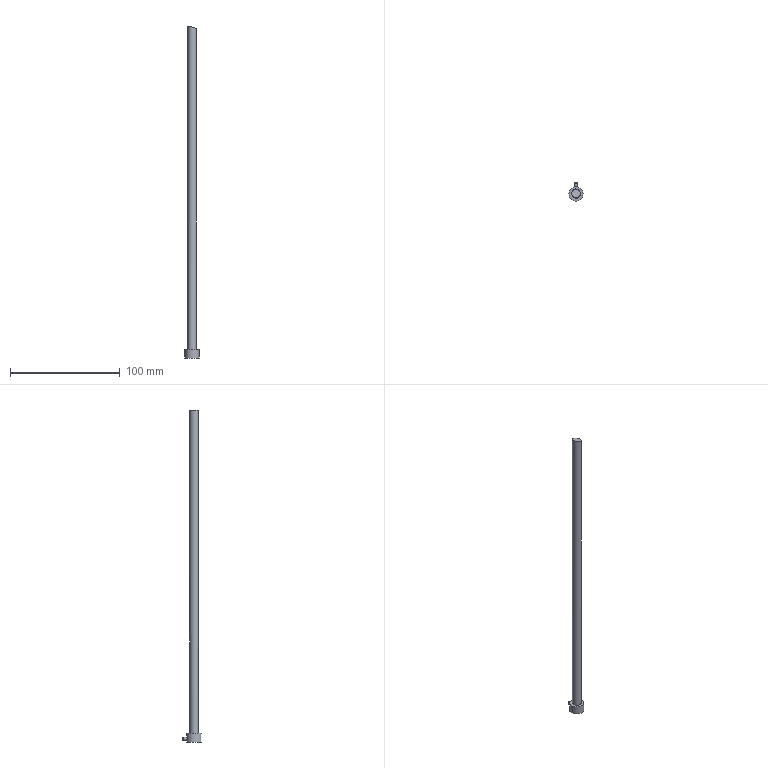Part | STEP file | E108-08-310 | 1 solid | 8 faces | box 13 x 16.5 x 302.869 mm | volume 15847 mm3 | cylinder 3 | plane 3 | spline 1 | cone 1 | commonest cylinder face diameters 3 x1 8 x1 13 x1
STEP:
#1=CARTESIAN_POINT('',(0.,0.,0.));
#2=DIRECTION('',(0.,0.,1.));
#3=DIRECTION('',(1.,0.,0.));
#4=AXIS2_PLACEMENT_3D('',#1,#2,#3);
#5=CARTESIAN_POINT('',(3.978,0.4166,300.445));
#6=VERTEX_POINT('',#5);
#7=CARTESIAN_POINT('',(3.978,0.4166,300.445));
#8=CARTESIAN_POINT('',(3.933,0.8473,300.446));
#9=CARTESIAN_POINT('',(3.815,1.276,300.47));
#10=CARTESIAN_POINT('',(3.636,1.668,300.514));
#11=CARTESIAN_POINT('',(3.456,2.059,300.558));
#12=CARTESIAN_POINT('',(3.21,2.424,300.623));
#13=CARTESIAN_POINT('',(2.92,2.734,300.703));
#14=CARTESIAN_POINT('',(2.623,3.051,300.785));
#15=CARTESIAN_POINT('',(2.272,3.319,300.885));
#16=CARTESIAN_POINT('',(1.896,3.522,300.994));
#17=CARTESIAN_POINT('',(1.503,3.734,301.108));
#18=CARTESIAN_POINT('',(1.071,3.879,301.235));
#19=CARTESIAN_POINT('',(0.6351,3.949,301.365));
#20=CARTESIAN_POINT('',(0.1817,4.022,301.5));
#21=CARTESIAN_POINT('',(-0.289,4.016,301.642));
#22=CARTESIAN_POINT('',(-0.7396,3.931,301.779));
#23=CARTESIAN_POINT('',(-1.199,3.845,301.92));
#24=CARTESIAN_POINT('',(-1.65,3.674,302.059));
#25=CARTESIAN_POINT('',(-2.054,3.432,302.186));
#26=CARTESIAN_POINT('',(-2.455,3.193,302.312));
#27=CARTESIAN_POINT('',(-2.82,2.876,302.43));
#28=CARTESIAN_POINT('',(-3.117,2.507,302.528));
#29=CARTESIAN_POINT('',(-3.404,2.15,302.623));
#30=CARTESIAN_POINT('',(-3.634,1.734,302.703));
#31=CARTESIAN_POINT('',(-3.785,1.295,302.76));
#32=CARTESIAN_POINT('',(-3.929,0.8741,302.815));
#33=CARTESIAN_POINT('',(-4.003,0.4197,302.851));
#34=CARTESIAN_POINT('',(-4.,-0.02828,302.863));
#35=CARTESIAN_POINT('',(-3.997,-0.4621,302.876));
#36=CARTESIAN_POINT('',(-3.921,-0.9021,302.867));
#37=CARTESIAN_POINT('',(-3.779,-1.311,302.838));
#38=CARTESIAN_POINT('',(-3.638,-1.717,302.809));
#39=CARTESIAN_POINT('',(-3.429,-2.103,302.76));
#40=CARTESIAN_POINT('',(-3.17,-2.44,302.694));
#41=CARTESIAN_POINT('',(-2.906,-2.782,302.627));
#42=CARTESIAN_POINT('',(-2.584,-3.083,302.541));
#43=CARTESIAN_POINT('',(-2.23,-3.32,302.444));
#44=CARTESIAN_POINT('',(-1.864,-3.567,302.343));
#45=CARTESIAN_POINT('',(-1.454,-3.752,302.227));
#46=CARTESIAN_POINT('',(-1.033,-3.864,302.104));
#47=CARTESIAN_POINT('',(-0.5946,-3.982,301.977));
#48=CARTESIAN_POINT('',(-0.1325,-4.023,301.839));
#49=CARTESIAN_POINT('',(0.317,-3.987,301.702));
#50=CARTESIAN_POINT('',(0.78,-3.951,301.561));
#51=CARTESIAN_POINT('',(1.242,-3.831,301.417));
#52=CARTESIAN_POINT('',(1.666,-3.636,301.282));
#53=CARTESIAN_POINT('',(2.092,-3.441,301.146));
#54=CARTESIAN_POINT('',(2.491,-3.165,301.015));
#55=CARTESIAN_POINT('',(2.827,-2.83,300.901));
#56=CARTESIAN_POINT('',(3.154,-2.503,300.79));
#57=CARTESIAN_POINT('',(3.431,-2.11,300.692));
#58=CARTESIAN_POINT('',(3.629,-1.683,300.618));
#59=CARTESIAN_POINT('',(3.818,-1.276,300.547));
#60=CARTESIAN_POINT('',(3.94,-0.8259,300.495));
#61=CARTESIAN_POINT('',(3.983,-0.3737,300.468));
#62=CARTESIAN_POINT('',(4.007,-0.1118,300.453));
#63=CARTESIAN_POINT('',(4.006,0.1545,300.445));
#64=CARTESIAN_POINT('',(3.978,0.4166,300.445));
#65=B_SPLINE_CURVE_WITH_KNOTS('',3,(#7,#8,#9,#10,#11,#12,#13,#14,#15,#16,#17,#18,#19,#20,#21,#22,#23,#24,#25,#26,#27,#28,#29,#30,#31,#32,#33,#34,#35,#36,#37,#38,#39,#40,#41,#42,#43,#44,#45,#46,#47,#48,#49,#50,#51,#52,#53,#54,#55,#56,#57,#58,#59,#60,#61,#62,#63,#64),.UNSPECIFIED.,.T.,.F.,(1,3,3,3,3,3,3,3,3,3,3,3,3,3,3,3,3,3,3,3,3,1),(-0.03062,0.,0.05078,0.1015,0.1532,0.2072,0.2634,0.3207,0.3775,0.4324,0.485,0.5359,0.5863,0.6375,0.6906,0.7458,0.8028,0.8601,0.916,0.9694,1.,1.051),.UNSPECIFIED.);
#66=CARTESIAN_POINT('',(0.,0.,108.));
#67=DIRECTION('',(0.,0.,-1.));
#68=DIRECTION('',(-1.,0.,0.));
#69=AXIS2_PLACEMENT_3D('',#66,#67,#68);
#70=CYLINDRICAL_SURFACE('',#69,4.);
#71=CARTESIAN_POINT('',(9.32,-192.445));
#72=CARTESIAN_POINT('',(9.296,-192.446));
#73=CARTESIAN_POINT('',(9.248,-192.448));
#74=CARTESIAN_POINT('',(9.174,-192.459));
#75=CARTESIAN_POINT('',(9.101,-192.476));
#76=CARTESIAN_POINT('',(9.029,-192.5));
#77=CARTESIAN_POINT('',(8.956,-192.529));
#78=CARTESIAN_POINT('',(8.884,-192.565));
#79=CARTESIAN_POINT('',(8.811,-192.607));
#80=CARTESIAN_POINT('',(8.739,-192.654));
#81=CARTESIAN_POINT('',(8.667,-192.706));
#82=CARTESIAN_POINT('',(8.596,-192.763));
#83=CARTESIAN_POINT('',(8.524,-192.824));
#84=CARTESIAN_POINT('',(8.453,-192.89));
#85=CARTESIAN_POINT('',(8.382,-192.959));
#86=CARTESIAN_POINT('',(8.311,-193.031));
#87=CARTESIAN_POINT('',(8.241,-193.106));
#88=CARTESIAN_POINT('',(8.17,-193.184));
#89=CARTESIAN_POINT('',(8.1,-193.264));
#90=CARTESIAN_POINT('',(8.03,-193.345));
#91=CARTESIAN_POINT('',(7.96,-193.427));
#92=CARTESIAN_POINT('',(7.89,-193.511));
#93=CARTESIAN_POINT('',(7.82,-193.596));
#94=CARTESIAN_POINT('',(7.75,-193.68));
#95=CARTESIAN_POINT('',(7.68,-193.765));
#96=CARTESIAN_POINT('',(7.611,-193.848));
#97=CARTESIAN_POINT('',(7.541,-193.931));
#98=CARTESIAN_POINT('',(7.471,-194.012));
#99=CARTESIAN_POINT('',(7.4,-194.092));
#100=CARTESIAN_POINT('',(7.33,-194.17));
#101=CARTESIAN_POINT('',(7.26,-194.245));
#102=CARTESIAN_POINT('',(7.189,-194.318));
#103=CARTESIAN_POINT('',(7.118,-194.387));
#104=CARTESIAN_POINT('',(7.047,-194.453));
#105=CARTESIAN_POINT('',(6.976,-194.516));
#106=CARTESIAN_POINT('',(6.905,-194.574));
#107=CARTESIAN_POINT('',(6.833,-194.627));
#108=CARTESIAN_POINT('',(6.761,-194.677));
#109=CARTESIAN_POINT('',(6.688,-194.721));
#110=CARTESIAN_POINT('',(6.616,-194.759));
#111=CARTESIAN_POINT('',(6.544,-194.792));
#112=CARTESIAN_POINT('',(6.471,-194.82));
#113=CARTESIAN_POINT('',(6.398,-194.842));
#114=CARTESIAN_POINT('',(6.325,-194.857));
#115=CARTESIAN_POINT('',(6.253,-194.867));
#116=CARTESIAN_POINT('',(6.18,-194.87));
#117=CARTESIAN_POINT('',(6.106,-194.867));
#118=CARTESIAN_POINT('',(6.033,-194.857));
#119=CARTESIAN_POINT('',(5.96,-194.842));
#120=CARTESIAN_POINT('',(5.888,-194.82));
#121=CARTESIAN_POINT('',(5.815,-194.793));
#122=CARTESIAN_POINT('',(5.742,-194.759));
#123=CARTESIAN_POINT('',(5.67,-194.72));
#124=CARTESIAN_POINT('',(5.598,-194.676));
#125=CARTESIAN_POINT('',(5.526,-194.627));
#126=CARTESIAN_POINT('',(5.454,-194.573));
#127=CARTESIAN_POINT('',(5.382,-194.514));
#128=CARTESIAN_POINT('',(5.311,-194.451));
#129=CARTESIAN_POINT('',(5.24,-194.385));
#130=CARTESIAN_POINT('',(5.169,-194.314));
#131=CARTESIAN_POINT('',(5.098,-194.241));
#132=CARTESIAN_POINT('',(5.028,-194.165));
#133=CARTESIAN_POINT('',(4.958,-194.087));
#134=CARTESIAN_POINT('',(4.887,-194.006));
#135=CARTESIAN_POINT('',(4.817,-193.924));
#136=CARTESIAN_POINT('',(4.747,-193.84));
#137=CARTESIAN_POINT('',(4.677,-193.756));
#138=CARTESIAN_POINT('',(4.608,-193.672));
#139=CARTESIAN_POINT('',(4.538,-193.587));
#140=CARTESIAN_POINT('',(4.468,-193.502));
#141=CARTESIAN_POINT('',(4.398,-193.417));
#142=CARTESIAN_POINT('',(4.328,-193.334));
#143=CARTESIAN_POINT('',(4.258,-193.253));
#144=CARTESIAN_POINT('',(4.188,-193.173));
#145=CARTESIAN_POINT('',(4.118,-193.095));
#146=CARTESIAN_POINT('',(4.047,-193.02));
#147=CARTESIAN_POINT('',(3.976,-192.948));
#148=CARTESIAN_POINT('',(3.906,-192.879));
#149=CARTESIAN_POINT('',(3.835,-192.814));
#150=CARTESIAN_POINT('',(3.763,-192.754));
#151=CARTESIAN_POINT('',(3.691,-192.697));
#152=CARTESIAN_POINT('',(3.619,-192.646));
#153=CARTESIAN_POINT('',(3.548,-192.6));
#154=CARTESIAN_POINT('',(3.475,-192.559));
#155=CARTESIAN_POINT('',(3.403,-192.524));
#156=CARTESIAN_POINT('',(3.33,-192.495));
#157=CARTESIAN_POINT('',(3.257,-192.473));
#158=CARTESIAN_POINT('',(3.184,-192.457));
#159=CARTESIAN_POINT('',(3.111,-192.447));
#160=CARTESIAN_POINT('',(3.062,-192.445));
#161=CARTESIAN_POINT('',(3.037,-192.445));
#162=B_SPLINE_CURVE_WITH_KNOTS('',3,(#71,#72,#73,#74,#75,#76,#77,#78,#79,#80,#81,#82,#83,#84,#85,#86,#87,#88,#89,#90,#91,#92,#93,#94,#95,#96,#97,#98,#99,#100,#101,#102,#103,#104,#105,#106,#107,#108,#109,#110,#111,#112,#113,#114,#115,#116,#117,#118,#119,#120,#121,#122,#123,#124,#125,#126,#127,#128,#129,#130,#131,#132,#133,#134,#135,#136,#137,#138,#139,#140,#141,#142,#143,#144,#145,#146,#147,#148,#149,#150,#151,#152,#153,#154,#155,#156,#157,#158,#159,#160,#161),.UNSPECIFIED.,.F.,.F.,(4,1,1,1,1,1,1,1,1,1,1,1,1,1,1,1,1,1,1,1,1,1,1,1,1,1,1,1,1,1,1,1,1,1,1,1,1,1,1,1,1,1,1,1,1,1,1,1,1,1,1,1,1,1,1,1,1,1,1,1,1,1,1,1,1,1,1,1,1,1,1,1,1,1,1,1,1,1,1,1,1,1,1,1,1,1,1,1,4),(0.,0.01136,0.02273,0.03409,0.04545,0.05682,0.06818,0.07955,0.09091,0.1023,0.1136,0.125,0.1364,0.1477,0.1591,0.1705,0.1818,0.1932,0.2045,0.2159,0.2273,0.2386,0.25,0.2614,0.2727,0.2841,0.2955,0.3068,0.3182,0.3295,0.3409,0.3523,0.3636,0.375,0.3864,0.3977,0.4091,0.4205,0.4318,0.4432,0.4545,0.4659,0.4773,0.4886,0.5,0.5114,0.5227,0.5341,0.5455,0.5568,0.5682,0.5795,0.5909,0.6023,0.6136,0.625,0.6364,0.6477,0.6591,0.6705,0.6818,0.6932,0.7045,0.7159,0.7273,0.7386,0.75,0.7614,0.7727,0.7841,0.7955,0.8068,0.8182,0.8295,0.8409,0.8523,0.8636,0.875,0.8864,0.8977,0.9091,0.9205,0.9318,0.9432,0.9545,0.9659,0.9773,0.9886,1.),.QUASI_UNIFORM_KNOTS.);
#163=(GEOMETRIC_REPRESENTATION_CONTEXT(2)PARAMETRIC_REPRESENTATION_CONTEXT()REPRESENTATION_CONTEXT('',''));
#164=DEFINITIONAL_REPRESENTATION('',(#162),#163);
#165=PCURVE('',#70,#164);
#166=CARTESIAN_POINT('',(-6.093,-7.25,303.685));
#167=CARTESIAN_POINT('',(-0.8456,-7.248,302.186));
#168=CARTESIAN_POINT('',(4.462,-7.246,300.56));
#169=CARTESIAN_POINT('',(9.83,-7.244,298.812));
#170=CARTESIAN_POINT('',(-6.112,-2.699,303.554));
#171=CARTESIAN_POINT('',(-0.8669,-2.697,302.056));
#172=CARTESIAN_POINT('',(4.438,-2.695,300.432));
#173=CARTESIAN_POINT('',(9.803,-2.692,298.685));
#174=CARTESIAN_POINT('',(-6.133,1.852,303.422));
#175=CARTESIAN_POINT('',(-0.8912,1.854,301.925));
#176=CARTESIAN_POINT('',(4.411,1.856,300.302));
#177=CARTESIAN_POINT('',(9.773,1.859,298.557));
#178=CARTESIAN_POINT('',(-6.157,6.403,303.288));
#179=CARTESIAN_POINT('',(-0.9182,6.405,301.793));
#180=CARTESIAN_POINT('',(4.381,6.407,300.171));
#181=CARTESIAN_POINT('',(9.741,6.409,298.427));
#182=B_SPLINE_SURFACE_WITH_KNOTS('',3,3,((#166,#167,#168,#169),(#170,#171,#172,#173),(#174,#175,#176,#177),(#178,#179,#180,#181)),.UNSPECIFIED.,.F.,.F.,.F.,(4,4),(4,4),(0.,1.),(0.,1.),.PIECEWISE_BEZIER_KNOTS.);
#183=CARTESIAN_POINT('',(0.5612,0.6378));
#184=CARTESIAN_POINT('',(0.5683,0.6372));
#185=CARTESIAN_POINT('',(0.5824,0.6356));
#186=CARTESIAN_POINT('',(0.6033,0.6318));
#187=CARTESIAN_POINT('',(0.6239,0.6267));
#188=CARTESIAN_POINT('',(0.6439,0.6204));
#189=CARTESIAN_POINT('',(0.6631,0.6129));
#190=CARTESIAN_POINT('',(0.6817,0.6042));
#191=CARTESIAN_POINT('',(0.6995,0.5943));
#192=CARTESIAN_POINT('',(0.7164,0.5834));
#193=CARTESIAN_POINT('',(0.7322,0.5716));
#194=CARTESIAN_POINT('',(0.7469,0.5589));
#195=CARTESIAN_POINT('',(0.7605,0.5453));
#196=CARTESIAN_POINT('',(0.7729,0.5309));
#197=CARTESIAN_POINT('',(0.7841,0.5158));
#198=CARTESIAN_POINT('',(0.7938,0.5003));
#199=CARTESIAN_POINT('',(0.8023,0.4841));
#200=CARTESIAN_POINT('',(0.8094,0.4675));
#201=CARTESIAN_POINT('',(0.8152,0.4505));
#202=CARTESIAN_POINT('',(0.8195,0.4332));
#203=CARTESIAN_POINT('',(0.8224,0.4159));
#204=CARTESIAN_POINT('',(0.8238,0.3983));
#205=CARTESIAN_POINT('',(0.8238,0.3806));
#206=CARTESIAN_POINT('',(0.8225,0.3629));
#207=CARTESIAN_POINT('',(0.8197,0.3455));
#208=CARTESIAN_POINT('',(0.8154,0.3283));
#209=CARTESIAN_POINT('',(0.8098,0.3112));
#210=CARTESIAN_POINT('',(0.8028,0.2945));
#211=CARTESIAN_POINT('',(0.7944,0.2782));
#212=CARTESIAN_POINT('',(0.7848,0.2625));
#213=CARTESIAN_POINT('',(0.7739,0.2474));
#214=CARTESIAN_POINT('',(0.7616,0.2329));
#215=CARTESIAN_POINT('',(0.7482,0.219));
#216=CARTESIAN_POINT('',(0.7337,0.206));
#217=CARTESIAN_POINT('',(0.7182,0.194));
#218=CARTESIAN_POINT('',(0.7016,0.1829));
#219=CARTESIAN_POINT('',(0.6841,0.1727));
#220=CARTESIAN_POINT('',(0.6657,0.1637));
#221=CARTESIAN_POINT('',(0.6465,0.1558));
#222=CARTESIAN_POINT('',(0.6268,0.149));
#223=CARTESIAN_POINT('',(0.6066,0.1436));
#224=CARTESIAN_POINT('',(0.5858,0.1394));
#225=CARTESIAN_POINT('',(0.5646,0.1365));
#226=CARTESIAN_POINT('',(0.5433,0.135));
#227=CARTESIAN_POINT('',(0.522,0.1348));
#228=CARTESIAN_POINT('',(0.5007,0.1359));
#229=CARTESIAN_POINT('',(0.4794,0.1384));
#230=CARTESIAN_POINT('',(0.4584,0.1423));
#231=CARTESIAN_POINT('',(0.4379,0.1474));
#232=CARTESIAN_POINT('',(0.418,0.1538));
#233=CARTESIAN_POINT('',(0.3986,0.1614));
#234=CARTESIAN_POINT('',(0.38,0.1703));
#235=CARTESIAN_POINT('',(0.3621,0.1802));
#236=CARTESIAN_POINT('',(0.3453,0.1911));
#237=CARTESIAN_POINT('',(0.3295,0.2031));
#238=CARTESIAN_POINT('',(0.3147,0.216));
#239=CARTESIAN_POINT('',(0.301,0.2298));
#240=CARTESIAN_POINT('',(0.2887,0.2442));
#241=CARTESIAN_POINT('',(0.2776,0.2594));
#242=CARTESIAN_POINT('',(0.2677,0.2751));
#243=CARTESIAN_POINT('',(0.2592,0.2915));
#244=CARTESIAN_POINT('',(0.2521,0.3082));
#245=CARTESIAN_POINT('',(0.2464,0.3252));
#246=CARTESIAN_POINT('',(0.2421,0.3424));
#247=CARTESIAN_POINT('',(0.2393,0.36));
#248=CARTESIAN_POINT('',(0.2378,0.3776));
#249=CARTESIAN_POINT('',(0.2378,0.3952));
#250=CARTESIAN_POINT('',(0.2392,0.4127));
#251=CARTESIAN_POINT('',(0.2421,0.4301));
#252=CARTESIAN_POINT('',(0.2463,0.4474));
#253=CARTESIAN_POINT('',(0.252,0.4644));
#254=CARTESIAN_POINT('',(0.259,0.4809));
#255=CARTESIAN_POINT('',(0.2673,0.497));
#256=CARTESIAN_POINT('',(0.277,0.5126));
#257=CARTESIAN_POINT('',(0.2879,0.5276));
#258=CARTESIAN_POINT('',(0.3001,0.5421));
#259=CARTESIAN_POINT('',(0.3135,0.5557));
#260=CARTESIAN_POINT('',(0.3279,0.5685));
#261=CARTESIAN_POINT('',(0.3434,0.5804));
#262=CARTESIAN_POINT('',(0.36,0.5915));
#263=CARTESIAN_POINT('',(0.3776,0.6015));
#264=CARTESIAN_POINT('',(0.3959,0.6105));
#265=CARTESIAN_POINT('',(0.4149,0.6183));
#266=CARTESIAN_POINT('',(0.4346,0.6249));
#267=CARTESIAN_POINT('',(0.455,0.6303));
#268=CARTESIAN_POINT('',(0.4758,0.6345));
#269=CARTESIAN_POINT('',(0.4968,0.6374));
#270=CARTESIAN_POINT('',(0.5182,0.639));
#271=CARTESIAN_POINT('',(0.5398,0.6392));
#272=CARTESIAN_POINT('',(0.5541,0.6384));
#273=CARTESIAN_POINT('',(0.5612,0.6378));
#274=B_SPLINE_CURVE_WITH_KNOTS('',3,(#183,#184,#185,#186,#187,#188,#189,#190,#191,#192,#193,#194,#195,#196,#197,#198,#199,#200,#201,#202,#203,#204,#205,#206,#207,#208,#209,#210,#211,#212,#213,#214,#215,#216,#217,#218,#219,#220,#221,#222,#223,#224,#225,#226,#227,#228,#229,#230,#231,#232,#233,#234,#235,#236,#237,#238,#239,#240,#241,#242,#243,#244,#245,#246,#247,#248,#249,#250,#251,#252,#253,#254,#255,#256,#257,#258,#259,#260,#261,#262,#263,#264,#265,#266,#267,#268,#269,#270,#271,#272,#273),.UNSPECIFIED.,.T.,.F.,(4,1,1,1,1,1,1,1,1,1,1,1,1,1,1,1,1,1,1,1,1,1,1,1,1,1,1,1,1,1,1,1,1,1,1,1,1,1,1,1,1,1,1,1,1,1,1,1,1,1,1,1,1,1,1,1,1,1,1,1,1,1,1,1,1,1,1,1,1,1,1,1,1,1,1,1,1,1,1,1,1,1,1,1,1,1,1,1,4),(0.,0.01136,0.02273,0.03409,0.04545,0.05682,0.06818,0.07955,0.09091,0.1023,0.1136,0.125,0.1364,0.1477,0.1591,0.1705,0.1818,0.1932,0.2045,0.2159,0.2273,0.2386,0.25,0.2614,0.2727,0.2841,0.2955,0.3068,0.3182,0.3295,0.3409,0.3523,0.3636,0.375,0.3864,0.3977,0.4091,0.4205,0.4318,0.4432,0.4545,0.4659,0.4773,0.4886,0.5,0.5114,0.5227,0.5341,0.5455,0.5568,0.5682,0.5795,0.5909,0.6023,0.6136,0.625,0.6364,0.6477,0.6591,0.6705,0.6818,0.6932,0.7045,0.7159,0.7273,0.7386,0.75,0.7614,0.7727,0.7841,0.7955,0.8068,0.8182,0.8295,0.8409,0.8523,0.8636,0.875,0.8864,0.8977,0.9091,0.9205,0.9318,0.9432,0.9545,0.9659,0.9773,0.9886,1.),.QUASI_UNIFORM_KNOTS.);
#275=(GEOMETRIC_REPRESENTATION_CONTEXT(2)PARAMETRIC_REPRESENTATION_CONTEXT()REPRESENTATION_CONTEXT('',''));
#276=DEFINITIONAL_REPRESENTATION('',(#274),#275);
#277=PCURVE('',#182,#276);
#278=SURFACE_CURVE('',#65,(#165,#277),.PCURVE_S1.);
#279=EDGE_CURVE('',#6,#6,#278,.T.);
#280=ORIENTED_EDGE('',*,*,#279,.F.);
#281=CARTESIAN_POINT('',(3.978,0.4166,8.));
#282=VERTEX_POINT('',#281);
#283=CARTESIAN_POINT('',(3.978,0.4166,300.445));
#284=CARTESIAN_POINT('',(3.978,0.4166,8.));
#285=B_SPLINE_CURVE_WITH_KNOTS('',1,(#283,#284),.UNSPECIFIED.,.F.,.F.,(2,2),(-192.445,100.),.PIECEWISE_BEZIER_KNOTS.);
#286=CARTESIAN_POINT('',(9.32,0.));
#287=DIRECTION('',(0.,1.));
#288=VECTOR('',#287,1.);
#289=LINE('',#286,#288);
#290=(GEOMETRIC_REPRESENTATION_CONTEXT(2)PARAMETRIC_REPRESENTATION_CONTEXT()REPRESENTATION_CONTEXT('',''));
#291=DEFINITIONAL_REPRESENTATION('',(#289),#290);
#292=PCURVE('',#70,#291);
#293=CARTESIAN_POINT('',(3.037,0.));
#294=DIRECTION('',(0.,1.));
#295=VECTOR('',#294,1.);
#296=LINE('',#293,#295);
#297=(GEOMETRIC_REPRESENTATION_CONTEXT(2)PARAMETRIC_REPRESENTATION_CONTEXT()REPRESENTATION_CONTEXT('',''));
#298=DEFINITIONAL_REPRESENTATION('',(#296),#297);
#299=PCURVE('',#70,#298);
#300=SEAM_CURVE('',#285,(#292,#299),.PCURVE_S1.);
#301=EDGE_CURVE('',#6,#282,#300,.T.);
#302=ORIENTED_EDGE('',*,*,#301,.T.);
#303=CARTESIAN_POINT('',(4.,0.,8.));
#304=VERTEX_POINT('',#303);
#305=CARTESIAN_POINT('',(0.,0.,8.));
#306=DIRECTION('',(0.,0.,1.));
#307=DIRECTION('',(1.,0.,0.));
#308=AXIS2_PLACEMENT_3D('',#305,#306,#307);
#309=CIRCLE('',#308,4.);
#310=CARTESIAN_POINT('',(9.425,100.));
#311=DIRECTION('',(-1.,0.));
#312=VECTOR('',#311,1.);
#313=LINE('',#310,#312);
#314=(GEOMETRIC_REPRESENTATION_CONTEXT(2)PARAMETRIC_REPRESENTATION_CONTEXT()REPRESENTATION_CONTEXT('',''));
#315=DEFINITIONAL_REPRESENTATION('',(#313),#314);
#316=PCURVE('',#70,#315);
#317=CARTESIAN_POINT('',(0.,0.,8.));
#318=DIRECTION('',(0.,0.,-1.));
#319=DIRECTION('',(1.,0.,0.));
#320=AXIS2_PLACEMENT_3D('',#317,#318,#319);
#321=PLANE('',#320);
#322=CARTESIAN_POINT('',(4.,0.));
#323=CARTESIAN_POINT('',(4.,-6.928));
#324=CARTESIAN_POINT('',(-2.,-3.464));
#325=CARTESIAN_POINT('',(-8.,0.));
#326=CARTESIAN_POINT('',(-2.,3.464));
#327=CARTESIAN_POINT('',(4.,6.928));
#328=CARTESIAN_POINT('',(4.,0.));
#329=(BOUNDED_CURVE()B_SPLINE_CURVE(2,(#322,#323,#324,#325,#326,#327,#328),.UNSPECIFIED.,.T.,.F.)B_SPLINE_CURVE_WITH_KNOTS((1,2,2,2,2,1),(-2.094,0.,2.094,4.189,6.283,8.378),.UNSPECIFIED.)CURVE()GEOMETRIC_REPRESENTATION_ITEM()RATIONAL_B_SPLINE_CURVE((1.,0.5,1.,0.5,1.,0.5,1.))REPRESENTATION_ITEM(''));
#330=(GEOMETRIC_REPRESENTATION_CONTEXT(2)PARAMETRIC_REPRESENTATION_CONTEXT()REPRESENTATION_CONTEXT('',''));
#331=DEFINITIONAL_REPRESENTATION('',(#329),#330);
#332=PCURVE('',#321,#331);
#333=SURFACE_CURVE('',#309,(#316,#332),.PCURVE_S1.);
#334=EDGE_CURVE('',#282,#304,#333,.T.);
#335=ORIENTED_EDGE('',*,*,#334,.T.);
#336=CARTESIAN_POINT('',(0.,0.,8.));
#337=DIRECTION('',(0.,0.,1.));
#338=DIRECTION('',(1.,0.,0.));
#339=AXIS2_PLACEMENT_3D('',#336,#337,#338);
#340=CIRCLE('',#339,4.);
#341=CARTESIAN_POINT('',(3.142,100.));
#342=DIRECTION('',(-1.,0.));
#343=VECTOR('',#342,1.);
#344=LINE('',#341,#343);
#345=(GEOMETRIC_REPRESENTATION_CONTEXT(2)PARAMETRIC_REPRESENTATION_CONTEXT()REPRESENTATION_CONTEXT('',''));
#346=DEFINITIONAL_REPRESENTATION('',(#344),#345);
#347=PCURVE('',#70,#346);
#348=CARTESIAN_POINT('',(4.,0.));
#349=CARTESIAN_POINT('',(4.,-6.928));
#350=CARTESIAN_POINT('',(-2.,-3.464));
#351=CARTESIAN_POINT('',(-8.,0.));
#352=CARTESIAN_POINT('',(-2.,3.464));
#353=CARTESIAN_POINT('',(4.,6.928));
#354=CARTESIAN_POINT('',(4.,0.));
#355=(BOUNDED_CURVE()B_SPLINE_CURVE(2,(#348,#349,#350,#351,#352,#353,#354),.UNSPECIFIED.,.T.,.F.)B_SPLINE_CURVE_WITH_KNOTS((1,2,2,2,2,1),(-2.094,0.,2.094,4.189,6.283,8.378),.UNSPECIFIED.)CURVE()GEOMETRIC_REPRESENTATION_ITEM()RATIONAL_B_SPLINE_CURVE((1.,0.5,1.,0.5,1.,0.5,1.))REPRESENTATION_ITEM(''));
#356=(GEOMETRIC_REPRESENTATION_CONTEXT(2)PARAMETRIC_REPRESENTATION_CONTEXT()REPRESENTATION_CONTEXT('',''));
#357=DEFINITIONAL_REPRESENTATION('',(#355),#356);
#358=PCURVE('',#321,#357);
#359=SURFACE_CURVE('',#340,(#347,#358),.PCURVE_S1.);
#360=EDGE_CURVE('',#304,#282,#359,.T.);
#361=ORIENTED_EDGE('',*,*,#360,.T.);
#362=ORIENTED_EDGE('',*,*,#301,.F.);
#363=EDGE_LOOP('',(#280,#302,#335,#361,#362));
#364=FACE_BOUND('',#363,.T.);
#365=ADVANCED_FACE('',(#364),#70,.T.);
#366=ORIENTED_EDGE('',*,*,#279,.F.);
#367=EDGE_LOOP('',(#366));
#368=FACE_BOUND('',#367,.F.);
#369=ADVANCED_FACE('',(#368),#182,.F.);
#370=CARTESIAN_POINT('',(6.5,0.,0.));
#371=VERTEX_POINT('',#370);
#372=CARTESIAN_POINT('',(-6.5,0.,0.));
#373=VERTEX_POINT('',#372);
#374=CARTESIAN_POINT('',(0.,0.,0.));
#375=DIRECTION('',(0.,0.,-1.));
#376=DIRECTION('',(-1.,0.,0.));
#377=AXIS2_PLACEMENT_3D('',#374,#375,#376);
#378=CIRCLE('',#377,6.5);
#379=CARTESIAN_POINT('',(0.,0.,8.));
#380=DIRECTION('',(0.,0.,-1.));
#381=DIRECTION('',(1.,0.,0.));
#382=AXIS2_PLACEMENT_3D('',#379,#380,#381);
#383=CYLINDRICAL_SURFACE('',#382,6.5);
#384=CARTESIAN_POINT('',(-3.142,8.));
#385=DIRECTION('',(1.,0.));
#386=VECTOR('',#385,1.);
#387=LINE('',#384,#386);
#388=(GEOMETRIC_REPRESENTATION_CONTEXT(2)PARAMETRIC_REPRESENTATION_CONTEXT()REPRESENTATION_CONTEXT('',''));
#389=DEFINITIONAL_REPRESENTATION('',(#387),#388);
#390=PCURVE('',#383,#389);
#391=CARTESIAN_POINT('',(240.,-1000.,0.));
#392=DIRECTION('',(0.,0.,1.));
#393=DIRECTION('',(-1.,0.,0.));
#394=AXIS2_PLACEMENT_3D('',#391,#392,#393);
#395=PLANE('',#394);
#396=CARTESIAN_POINT('',(246.5,-1000.));
#397=CARTESIAN_POINT('',(246.5,-1011.258));
#398=CARTESIAN_POINT('',(236.75,-1005.629));
#399=CARTESIAN_POINT('',(227.,-1000.));
#400=CARTESIAN_POINT('',(236.75,-994.371));
#401=CARTESIAN_POINT('',(246.5,-988.742));
#402=CARTESIAN_POINT('',(246.5,-1000.));
#403=(BOUNDED_CURVE()B_SPLINE_CURVE(2,(#396,#397,#398,#399,#400,#401,#402),.UNSPECIFIED.,.T.,.F.)B_SPLINE_CURVE_WITH_KNOTS((1,2,2,2,2,1),(-2.094,0.,2.094,4.189,6.283,8.378),.UNSPECIFIED.)CURVE()GEOMETRIC_REPRESENTATION_ITEM()RATIONAL_B_SPLINE_CURVE((1.,0.5,1.,0.5,1.,0.5,1.))REPRESENTATION_ITEM(''));
#404=(GEOMETRIC_REPRESENTATION_CONTEXT(2)PARAMETRIC_REPRESENTATION_CONTEXT()REPRESENTATION_CONTEXT('',''));
#405=DEFINITIONAL_REPRESENTATION('',(#403),#404);
#406=PCURVE('',#395,#405);
#407=SURFACE_CURVE('',#378,(#390,#406),.PCURVE_S1.);
#408=EDGE_CURVE('',#371,#373,#407,.T.);
#409=ORIENTED_EDGE('',*,*,#408,.F.);
#410=CARTESIAN_POINT('',(6.5,0.,8.));
#411=VERTEX_POINT('',#410);
#412=CARTESIAN_POINT('',(6.5,0.,8.));
#413=CARTESIAN_POINT('',(6.5,0.,0.));
#414=B_SPLINE_CURVE_WITH_KNOTS('',1,(#412,#413),.UNSPECIFIED.,.F.,.F.,(2,2),(0.,8.),.PIECEWISE_BEZIER_KNOTS.);
#415=CARTESIAN_POINT('',(0.,0.));
#416=DIRECTION('',(0.,1.));
#417=VECTOR('',#416,1.);
#418=LINE('',#415,#417);
#419=(GEOMETRIC_REPRESENTATION_CONTEXT(2)PARAMETRIC_REPRESENTATION_CONTEXT()REPRESENTATION_CONTEXT('',''));
#420=DEFINITIONAL_REPRESENTATION('',(#418),#419);
#421=PCURVE('',#383,#420);
#422=CARTESIAN_POINT('',(6.283,0.));
#423=DIRECTION('',(0.,1.));
#424=VECTOR('',#423,1.);
#425=LINE('',#422,#424);
#426=(GEOMETRIC_REPRESENTATION_CONTEXT(2)PARAMETRIC_REPRESENTATION_CONTEXT()REPRESENTATION_CONTEXT('',''));
#427=DEFINITIONAL_REPRESENTATION('',(#425),#426);
#428=PCURVE('',#383,#427);
#429=SEAM_CURVE('',#414,(#421,#428),.PCURVE_S1.);
#430=EDGE_CURVE('',#411,#371,#429,.T.);
#431=ORIENTED_EDGE('',*,*,#430,.F.);
#432=CARTESIAN_POINT('',(0.,0.,8.));
#433=DIRECTION('',(0.,0.,-1.));
#434=DIRECTION('',(1.,0.,0.));
#435=AXIS2_PLACEMENT_3D('',#432,#433,#434);
#436=CIRCLE('',#435,6.5);
#437=CARTESIAN_POINT('',(0.,0.));
#438=DIRECTION('',(1.,0.));
#439=VECTOR('',#438,1.);
#440=LINE('',#437,#439);
#441=(GEOMETRIC_REPRESENTATION_CONTEXT(2)PARAMETRIC_REPRESENTATION_CONTEXT()REPRESENTATION_CONTEXT('',''));
#442=DEFINITIONAL_REPRESENTATION('',(#440),#441);
#443=PCURVE('',#383,#442);
#444=CARTESIAN_POINT('',(0.,0.));
#445=DIRECTION('',(1.,0.));
#446=AXIS2_PLACEMENT_2D('',#444,#445);
#447=CIRCLE('',#446,6.5);
#448=(GEOMETRIC_REPRESENTATION_CONTEXT(2)PARAMETRIC_REPRESENTATION_CONTEXT()REPRESENTATION_CONTEXT('',''));
#449=DEFINITIONAL_REPRESENTATION('',(#447),#448);
#450=PCURVE('',#321,#449);
#451=SURFACE_CURVE('',#436,(#443,#450),.PCURVE_S1.);
#452=EDGE_CURVE('',#411,#411,#451,.T.);
#453=ORIENTED_EDGE('',*,*,#452,.T.);
#454=ORIENTED_EDGE('',*,*,#430,.T.);
#455=CARTESIAN_POINT('',(0.,0.,0.));
#456=DIRECTION('',(0.,0.,-1.));
#457=DIRECTION('',(-1.,0.,0.));
#458=AXIS2_PLACEMENT_3D('',#455,#456,#457);
#459=CIRCLE('',#458,6.5);
#460=CARTESIAN_POINT('',(3.142,8.));
#461=DIRECTION('',(1.,0.));
#462=VECTOR('',#461,1.);
#463=LINE('',#460,#462);
#464=(GEOMETRIC_REPRESENTATION_CONTEXT(2)PARAMETRIC_REPRESENTATION_CONTEXT()REPRESENTATION_CONTEXT('',''));
#465=DEFINITIONAL_REPRESENTATION('',(#463),#464);
#466=PCURVE('',#383,#465);
#467=CARTESIAN_POINT('',(246.5,-1000.));
#468=CARTESIAN_POINT('',(246.5,-1011.258));
#469=CARTESIAN_POINT('',(236.75,-1005.629));
#470=CARTESIAN_POINT('',(227.,-1000.));
#471=CARTESIAN_POINT('',(236.75,-994.371));
#472=CARTESIAN_POINT('',(246.5,-988.742));
#473=CARTESIAN_POINT('',(246.5,-1000.));
#474=(BOUNDED_CURVE()B_SPLINE_CURVE(2,(#467,#468,#469,#470,#471,#472,#473),.UNSPECIFIED.,.T.,.F.)B_SPLINE_CURVE_WITH_KNOTS((1,2,2,2,2,1),(-2.094,0.,2.094,4.189,6.283,8.378),.UNSPECIFIED.)CURVE()GEOMETRIC_REPRESENTATION_ITEM()RATIONAL_B_SPLINE_CURVE((1.,0.5,1.,0.5,1.,0.5,1.))REPRESENTATION_ITEM(''));
#475=(GEOMETRIC_REPRESENTATION_CONTEXT(2)PARAMETRIC_REPRESENTATION_CONTEXT()REPRESENTATION_CONTEXT('',''));
#476=DEFINITIONAL_REPRESENTATION('',(#474),#475);
#477=PCURVE('',#395,#476);
#478=SURFACE_CURVE('',#459,(#466,#477),.PCURVE_S1.);
#479=EDGE_CURVE('',#373,#371,#478,.T.);
#480=ORIENTED_EDGE('',*,*,#479,.F.);
#481=EDGE_LOOP('',(#409,#431,#453,#454,#480));
#482=FACE_BOUND('',#481,.T.);
#483=CARTESIAN_POINT('',(0.,6.5,1.5));
#484=VERTEX_POINT('',#483);
#485=CARTESIAN_POINT('',(0.,6.5,1.5));
#486=CARTESIAN_POINT('',(0.1654,6.5,1.5));
#487=CARTESIAN_POINT('',(0.3332,6.493,1.528));
#488=CARTESIAN_POINT('',(0.4892,6.482,1.582));
#489=CARTESIAN_POINT('',(0.6451,6.47,1.636));
#490=CARTESIAN_POINT('',(0.7936,6.453,1.717));
#491=CARTESIAN_POINT('',(0.9231,6.434,1.818));
#492=CARTESIAN_POINT('',(1.055,6.415,1.92));
#493=CARTESIAN_POINT('',(1.17,6.394,2.047));
#494=CARTESIAN_POINT('',(1.261,6.377,2.187));
#495=CARTESIAN_POINT('',(1.352,6.358,2.329));
#496=CARTESIAN_POINT('',(1.421,6.343,2.49));
#497=CARTESIAN_POINT('',(1.46,6.334,2.655));
#498=CARTESIAN_POINT('',(1.498,6.325,2.817));
#499=CARTESIAN_POINT('',(1.509,6.322,2.989));
#500=CARTESIAN_POINT('',(1.492,6.326,3.155));
#501=CARTESIAN_POINT('',(1.475,6.33,3.318));
#502=CARTESIAN_POINT('',(1.431,6.341,3.48));
#503=CARTESIAN_POINT('',(1.362,6.356,3.628));
#504=CARTESIAN_POINT('',(1.293,6.37,3.777));
#505=CARTESIAN_POINT('',(1.199,6.39,3.917));
#506=CARTESIAN_POINT('',(1.085,6.409,4.035));
#507=CARTESIAN_POINT('',(0.9695,6.428,4.157));
#508=CARTESIAN_POINT('',(0.8309,6.448,4.26));
#509=CARTESIAN_POINT('',(0.6809,6.464,4.337));
#510=CARTESIAN_POINT('',(0.5305,6.48,4.413));
#511=CARTESIAN_POINT('',(0.3642,6.492,4.465));
#512=CARTESIAN_POINT('',(0.1962,6.497,4.487));
#513=CARTESIAN_POINT('',(0.03191,6.502,4.509));
#514=CARTESIAN_POINT('',(-0.1386,6.501,4.503));
#515=CARTESIAN_POINT('',(-0.3008,6.493,4.47));
#516=CARTESIAN_POINT('',(-0.4611,6.486,4.437));
#517=CARTESIAN_POINT('',(-0.6177,6.472,4.377));
#518=CARTESIAN_POINT('',(-0.7583,6.456,4.294));
#519=CARTESIAN_POINT('',(-0.9011,6.439,4.211));
#520=CARTESIAN_POINT('',(-1.031,6.419,4.102));
#521=CARTESIAN_POINT('',(-1.139,6.399,3.976));
#522=CARTESIAN_POINT('',(-1.249,6.38,3.848));
#523=CARTESIAN_POINT('',(-1.338,6.361,3.699));
#524=CARTESIAN_POINT('',(-1.399,6.348,3.541));
#525=CARTESIAN_POINT('',(-1.46,6.334,3.384));
#526=CARTESIAN_POINT('',(-1.494,6.326,3.214));
#527=CARTESIAN_POINT('',(-1.499,6.325,3.046));
#528=CARTESIAN_POINT('',(-1.504,6.324,2.881));
#529=CARTESIAN_POINT('',(-1.482,6.329,2.714));
#530=CARTESIAN_POINT('',(-1.433,6.34,2.557));
#531=CARTESIAN_POINT('',(-1.385,6.351,2.4));
#532=CARTESIAN_POINT('',(-1.309,6.367,2.25));
#533=CARTESIAN_POINT('',(-1.214,6.386,2.119));
#534=CARTESIAN_POINT('',(-1.116,6.404,1.984));
#535=CARTESIAN_POINT('',(-0.9937,6.425,1.864));
#536=CARTESIAN_POINT('',(-0.8569,6.443,1.769));
#537=CARTESIAN_POINT('',(-0.7182,6.462,1.672));
#538=CARTESIAN_POINT('',(-0.5604,6.478,1.598));
#539=CARTESIAN_POINT('',(-0.3967,6.488,1.553));
#540=CARTESIAN_POINT('',(-0.2682,6.496,1.518));
#541=CARTESIAN_POINT('',(-0.1335,6.5,1.5));
#542=CARTESIAN_POINT('',(0.,6.5,1.5));
#543=B_SPLINE_CURVE_WITH_KNOTS('',3,(#485,#486,#487,#488,#489,#490,#491,#492,#493,#494,#495,#496,#497,#498,#499,#500,#501,#502,#503,#504,#505,#506,#507,#508,#509,#510,#511,#512,#513,#514,#515,#516,#517,#518,#519,#520,#521,#522,#523,#524,#525,#526,#527,#528,#529,#530,#531,#532,#533,#534,#535,#536,#537,#538,#539,#540,#541,#542),.UNSPECIFIED.,.T.,.F.,(1,3,3,3,3,3,3,3,3,3,3,3,3,3,3,3,3,3,3,3,3,1),(-0.04234,0.,0.05275,0.1054,0.159,0.2132,0.2665,0.3187,0.3713,0.4252,0.4793,0.5321,0.5843,0.6373,0.6915,0.7453,0.7978,0.85,0.9034,0.9577,1.,1.053),.UNSPECIFIED.);
#544=CARTESIAN_POINT('',(4.712,6.5));
#545=CARTESIAN_POINT('',(4.718,6.5));
#546=CARTESIAN_POINT('',(4.729,6.497));
#547=CARTESIAN_POINT('',(4.745,6.486));
#548=CARTESIAN_POINT('',(4.762,6.467));
#549=CARTESIAN_POINT('',(4.778,6.44));
#550=CARTESIAN_POINT('',(4.793,6.406));
#551=CARTESIAN_POINT('',(4.809,6.365));
#552=CARTESIAN_POINT('',(4.823,6.317));
#553=CARTESIAN_POINT('',(4.838,6.262));
#554=CARTESIAN_POINT('',(4.851,6.201));
#555=CARTESIAN_POINT('',(4.864,6.135));
#556=CARTESIAN_POINT('',(4.876,6.062));
#557=CARTESIAN_POINT('',(4.888,5.983));
#558=CARTESIAN_POINT('',(4.898,5.9));
#559=CARTESIAN_POINT('',(4.908,5.813));
#560=CARTESIAN_POINT('',(4.916,5.721));
#561=CARTESIAN_POINT('',(4.924,5.625));
#562=CARTESIAN_POINT('',(4.93,5.526));
#563=CARTESIAN_POINT('',(4.936,5.424));
#564=CARTESIAN_POINT('',(4.94,5.321));
#565=CARTESIAN_POINT('',(4.943,5.215));
#566=CARTESIAN_POINT('',(4.945,5.108));
#567=CARTESIAN_POINT('',(4.945,5.));
#568=CARTESIAN_POINT('',(4.945,4.893));
#569=CARTESIAN_POINT('',(4.943,4.787));
#570=CARTESIAN_POINT('',(4.94,4.681));
#571=CARTESIAN_POINT('',(4.936,4.576));
#572=CARTESIAN_POINT('',(4.93,4.474));
#573=CARTESIAN_POINT('',(4.924,4.376));
#574=CARTESIAN_POINT('',(4.916,4.28));
#575=CARTESIAN_POINT('',(4.908,4.188));
#576=CARTESIAN_POINT('',(4.898,4.1));
#577=CARTESIAN_POINT('',(4.888,4.017));
#578=CARTESIAN_POINT('',(4.877,3.939));
#579=CARTESIAN_POINT('',(4.864,3.866));
#580=CARTESIAN_POINT('',(4.851,3.799));
#581=CARTESIAN_POINT('',(4.838,3.738));
#582=CARTESIAN_POINT('',(4.824,3.683));
#583=CARTESIAN_POINT('',(4.809,3.635));
#584=CARTESIAN_POINT('',(4.793,3.594));
#585=CARTESIAN_POINT('',(4.778,3.56));
#586=CARTESIAN_POINT('',(4.762,3.533));
#587=CARTESIAN_POINT('',(4.745,3.514));
#588=CARTESIAN_POINT('',(4.729,3.503));
#589=CARTESIAN_POINT('',(4.713,3.499));
#590=CARTESIAN_POINT('',(4.696,3.503));
#591=CARTESIAN_POINT('',(4.679,3.514));
#592=CARTESIAN_POINT('',(4.663,3.533));
#593=CARTESIAN_POINT('',(4.647,3.56));
#594=CARTESIAN_POINT('',(4.632,3.594));
#595=CARTESIAN_POINT('',(4.616,3.635));
#596=CARTESIAN_POINT('',(4.601,3.683));
#597=CARTESIAN_POINT('',(4.587,3.737));
#598=CARTESIAN_POINT('',(4.574,3.798));
#599=CARTESIAN_POINT('',(4.561,3.865));
#600=CARTESIAN_POINT('',(4.548,3.938));
#601=CARTESIAN_POINT('',(4.537,4.016));
#602=CARTESIAN_POINT('',(4.527,4.099));
#603=CARTESIAN_POINT('',(4.517,4.187));
#604=CARTESIAN_POINT('',(4.508,4.279));
#605=CARTESIAN_POINT('',(4.501,4.375));
#606=CARTESIAN_POINT('',(4.494,4.473));
#607=CARTESIAN_POINT('',(4.489,4.575));
#608=CARTESIAN_POINT('',(4.485,4.679));
#609=CARTESIAN_POINT('',(4.482,4.785));
#610=CARTESIAN_POINT('',(4.48,4.892));
#611=CARTESIAN_POINT('',(4.479,4.999));
#612=CARTESIAN_POINT('',(4.48,5.106));
#613=CARTESIAN_POINT('',(4.482,5.213));
#614=CARTESIAN_POINT('',(4.485,5.319));
#615=CARTESIAN_POINT('',(4.489,5.423));
#616=CARTESIAN_POINT('',(4.494,5.524));
#617=CARTESIAN_POINT('',(4.501,5.624));
#618=CARTESIAN_POINT('',(4.508,5.72));
#619=CARTESIAN_POINT('',(4.517,5.812));
#620=CARTESIAN_POINT('',(4.526,5.899));
#621=CARTESIAN_POINT('',(4.537,5.982));
#622=CARTESIAN_POINT('',(4.548,6.061));
#623=CARTESIAN_POINT('',(4.56,6.134));
#624=CARTESIAN_POINT('',(4.573,6.201));
#625=CARTESIAN_POINT('',(4.587,6.262));
#626=CARTESIAN_POINT('',(4.601,6.316));
#627=CARTESIAN_POINT('',(4.616,6.364));
#628=CARTESIAN_POINT('',(4.631,6.406));
#629=CARTESIAN_POINT('',(4.647,6.44));
#630=CARTESIAN_POINT('',(4.663,6.466));
#631=CARTESIAN_POINT('',(4.679,6.486));
#632=CARTESIAN_POINT('',(4.696,6.497));
#633=CARTESIAN_POINT('',(4.707,6.5));
#634=CARTESIAN_POINT('',(4.712,6.5));
#635=B_SPLINE_CURVE_WITH_KNOTS('',3,(#544,#545,#546,#547,#548,#549,#550,#551,#552,#553,#554,#555,#556,#557,#558,#559,#560,#561,#562,#563,#564,#565,#566,#567,#568,#569,#570,#571,#572,#573,#574,#575,#576,#577,#578,#579,#580,#581,#582,#583,#584,#585,#586,#587,#588,#589,#590,#591,#592,#593,#594,#595,#596,#597,#598,#599,#600,#601,#602,#603,#604,#605,#606,#607,#608,#609,#610,#611,#612,#613,#614,#615,#616,#617,#618,#619,#620,#621,#622,#623,#624,#625,#626,#627,#628,#629,#630,#631,#632,#633,#634),.UNSPECIFIED.,.T.,.F.,(4,1,1,1,1,1,1,1,1,1,1,1,1,1,1,1,1,1,1,1,1,1,1,1,1,1,1,1,1,1,1,1,1,1,1,1,1,1,1,1,1,1,1,1,1,1,1,1,1,1,1,1,1,1,1,1,1,1,1,1,1,1,1,1,1,1,1,1,1,1,1,1,1,1,1,1,1,1,1,1,1,1,1,1,1,1,1,1,4),(0.,0.01136,0.02273,0.03409,0.04545,0.05682,0.06818,0.07955,0.09091,0.1023,0.1136,0.125,0.1364,0.1477,0.1591,0.1705,0.1818,0.1932,0.2045,0.2159,0.2273,0.2386,0.25,0.2614,0.2727,0.2841,0.2955,0.3068,0.3182,0.3295,0.3409,0.3523,0.3636,0.375,0.3864,0.3977,0.4091,0.4205,0.4318,0.4432,0.4545,0.4659,0.4773,0.4886,0.5,0.5114,0.5227,0.5341,0.5455,0.5568,0.5682,0.5795,0.5909,0.6023,0.6136,0.625,0.6364,0.6477,0.6591,0.6705,0.6818,0.6932,0.7045,0.7159,0.7273,0.7386,0.75,0.7614,0.7727,0.7841,0.7955,0.8068,0.8182,0.8295,0.8409,0.8523,0.8636,0.875,0.8864,0.8977,0.9091,0.9205,0.9318,0.9432,0.9545,0.9659,0.9773,0.9886,1.),.QUASI_UNIFORM_KNOTS.);
#636=(GEOMETRIC_REPRESENTATION_CONTEXT(2)PARAMETRIC_REPRESENTATION_CONTEXT()REPRESENTATION_CONTEXT('',''));
#637=DEFINITIONAL_REPRESENTATION('',(#635),#636);
#638=PCURVE('',#383,#637);
#639=CARTESIAN_POINT('',(0.,2.,3.));
#640=DIRECTION('',(0.,1.,0.));
#641=DIRECTION('',(0.,0.,-1.));
#642=AXIS2_PLACEMENT_3D('',#639,#640,#641);
#643=CYLINDRICAL_SURFACE('',#642,1.5);
#644=CARTESIAN_POINT('',(6.283,4.5));
#645=CARTESIAN_POINT('',(6.259,4.5));
#646=CARTESIAN_POINT('',(6.212,4.499));
#647=CARTESIAN_POINT('',(6.14,4.497));
#648=CARTESIAN_POINT('',(6.068,4.492));
#649=CARTESIAN_POINT('',(5.997,4.486));
#650=CARTESIAN_POINT('',(5.926,4.479));
#651=CARTESIAN_POINT('',(5.854,4.47));
#652=CARTESIAN_POINT('',(5.783,4.46));
#653=CARTESIAN_POINT('',(5.711,4.449));
#654=CARTESIAN_POINT('',(5.64,4.438));
#655=CARTESIAN_POINT('',(5.569,4.425));
#656=CARTESIAN_POINT('',(5.498,4.413));
#657=CARTESIAN_POINT('',(5.427,4.4));
#658=CARTESIAN_POINT('',(5.355,4.388));
#659=CARTESIAN_POINT('',(5.284,4.376));
#660=CARTESIAN_POINT('',(5.213,4.365));
#661=CARTESIAN_POINT('',(5.142,4.355));
#662=CARTESIAN_POINT('',(5.07,4.346));
#663=CARTESIAN_POINT('',(4.999,4.338));
#664=CARTESIAN_POINT('',(4.928,4.332));
#665=CARTESIAN_POINT('',(4.856,4.328));
#666=CARTESIAN_POINT('',(4.784,4.325));
#667=CARTESIAN_POINT('',(4.713,4.324));
#668=CARTESIAN_POINT('',(4.641,4.325));
#669=CARTESIAN_POINT('',(4.57,4.328));
#670=CARTESIAN_POINT('',(4.498,4.332));
#671=CARTESIAN_POINT('',(4.426,4.339));
#672=CARTESIAN_POINT('',(4.355,4.346));
#673=CARTESIAN_POINT('',(4.283,4.355));
#674=CARTESIAN_POINT('',(4.212,4.365));
#675=CARTESIAN_POINT('',(4.141,4.376));
#676=CARTESIAN_POINT('',(4.07,4.388));
#677=CARTESIAN_POINT('',(3.998,4.4));
#678=CARTESIAN_POINT('',(3.927,4.413));
#679=CARTESIAN_POINT('',(3.856,4.425));
#680=CARTESIAN_POINT('',(3.785,4.437));
#681=CARTESIAN_POINT('',(3.714,4.449));
#682=CARTESIAN_POINT('',(3.642,4.46));
#683=CARTESIAN_POINT('',(3.571,4.47));
#684=CARTESIAN_POINT('',(3.5,4.479));
#685=CARTESIAN_POINT('',(3.428,4.486));
#686=CARTESIAN_POINT('',(3.357,4.492));
#687=CARTESIAN_POINT('',(3.285,4.497));
#688=CARTESIAN_POINT('',(3.214,4.499));
#689=CARTESIAN_POINT('',(3.142,4.5));
#690=CARTESIAN_POINT('',(3.07,4.499));
#691=CARTESIAN_POINT('',(2.999,4.497));
#692=CARTESIAN_POINT('',(2.927,4.492));
#693=CARTESIAN_POINT('',(2.856,4.486));
#694=CARTESIAN_POINT('',(2.784,4.479));
#695=CARTESIAN_POINT('',(2.713,4.47));
#696=CARTESIAN_POINT('',(2.641,4.46));
#697=CARTESIAN_POINT('',(2.57,4.449));
#698=CARTESIAN_POINT('',(2.499,4.438));
#699=CARTESIAN_POINT('',(2.428,4.425));
#700=CARTESIAN_POINT('',(2.357,4.413));
#701=CARTESIAN_POINT('',(2.285,4.4));
#702=CARTESIAN_POINT('',(2.215,4.388));
#703=CARTESIAN_POINT('',(2.143,4.376));
#704=CARTESIAN_POINT('',(2.072,4.365));
#705=CARTESIAN_POINT('',(2.,4.355));
#706=CARTESIAN_POINT('',(1.929,4.346));
#707=CARTESIAN_POINT('',(1.858,4.339));
#708=CARTESIAN_POINT('',(1.786,4.332));
#709=CARTESIAN_POINT('',(1.715,4.328));
#710=CARTESIAN_POINT('',(1.643,4.325));
#711=CARTESIAN_POINT('',(1.572,4.324));
#712=CARTESIAN_POINT('',(1.5,4.325));
#713=CARTESIAN_POINT('',(1.428,4.328));
#714=CARTESIAN_POINT('',(1.357,4.332));
#715=CARTESIAN_POINT('',(1.285,4.338));
#716=CARTESIAN_POINT('',(1.214,4.346));
#717=CARTESIAN_POINT('',(1.142,4.355));
#718=CARTESIAN_POINT('',(1.071,4.365));
#719=CARTESIAN_POINT('',(0.9995,4.376));
#720=CARTESIAN_POINT('',(0.9286,4.388));
#721=CARTESIAN_POINT('',(0.8575,4.4));
#722=CARTESIAN_POINT('',(0.7862,4.413));
#723=CARTESIAN_POINT('',(0.7149,4.425));
#724=CARTESIAN_POINT('',(0.6436,4.437));
#725=CARTESIAN_POINT('',(0.5728,4.449));
#726=CARTESIAN_POINT('',(0.5015,4.46));
#727=CARTESIAN_POINT('',(0.43,4.47));
#728=CARTESIAN_POINT('',(0.3585,4.479));
#729=CARTESIAN_POINT('',(0.2872,4.486));
#730=CARTESIAN_POINT('',(0.2157,4.492));
#731=CARTESIAN_POINT('',(0.1438,4.497));
#732=CARTESIAN_POINT('',(0.07178,4.499));
#733=CARTESIAN_POINT('',(0.02388,4.5));
#734=CARTESIAN_POINT('',(0.,4.5));
#735=B_SPLINE_CURVE_WITH_KNOTS('',3,(#644,#645,#646,#647,#648,#649,#650,#651,#652,#653,#654,#655,#656,#657,#658,#659,#660,#661,#662,#663,#664,#665,#666,#667,#668,#669,#670,#671,#672,#673,#674,#675,#676,#677,#678,#679,#680,#681,#682,#683,#684,#685,#686,#687,#688,#689,#690,#691,#692,#693,#694,#695,#696,#697,#698,#699,#700,#701,#702,#703,#704,#705,#706,#707,#708,#709,#710,#711,#712,#713,#714,#715,#716,#717,#718,#719,#720,#721,#722,#723,#724,#725,#726,#727,#728,#729,#730,#731,#732,#733,#734),.UNSPECIFIED.,.F.,.F.,(4,1,1,1,1,1,1,1,1,1,1,1,1,1,1,1,1,1,1,1,1,1,1,1,1,1,1,1,1,1,1,1,1,1,1,1,1,1,1,1,1,1,1,1,1,1,1,1,1,1,1,1,1,1,1,1,1,1,1,1,1,1,1,1,1,1,1,1,1,1,1,1,1,1,1,1,1,1,1,1,1,1,1,1,1,1,1,1,4),(0.,0.01136,0.02273,0.03409,0.04545,0.05682,0.06818,0.07955,0.09091,0.1023,0.1136,0.125,0.1364,0.1477,0.1591,0.1705,0.1818,0.1932,0.2045,0.2159,0.2273,0.2386,0.25,0.2614,0.2727,0.2841,0.2955,0.3068,0.3182,0.3295,0.3409,0.3523,0.3636,0.375,0.3864,0.3977,0.4091,0.4205,0.4318,0.4432,0.4545,0.4659,0.4773,0.4886,0.5,0.5114,0.5227,0.5341,0.5455,0.5568,0.5682,0.5795,0.5909,0.6023,0.6136,0.625,0.6364,0.6477,0.6591,0.6705,0.6818,0.6932,0.7045,0.7159,0.7273,0.7386,0.75,0.7614,0.7727,0.7841,0.7955,0.8068,0.8182,0.8295,0.8409,0.8523,0.8636,0.875,0.8864,0.8977,0.9091,0.9205,0.9318,0.9432,0.9545,0.9659,0.9773,0.9886,1.),.QUASI_UNIFORM_KNOTS.);
#736=(GEOMETRIC_REPRESENTATION_CONTEXT(2)PARAMETRIC_REPRESENTATION_CONTEXT()REPRESENTATION_CONTEXT('',''));
#737=DEFINITIONAL_REPRESENTATION('',(#735),#736);
#738=PCURVE('',#643,#737);
#739=SURFACE_CURVE('',#543,(#638,#738),.PCURVE_S1.);
#740=EDGE_CURVE('',#484,#484,#739,.T.);
#741=ORIENTED_EDGE('',*,*,#740,.T.);
#742=EDGE_LOOP('',(#741));
#743=FACE_BOUND('',#742,.T.);
#744=ADVANCED_FACE('',(#482,#743),#383,.T.);
#745=ORIENTED_EDGE('',*,*,#360,.F.);
#746=ORIENTED_EDGE('',*,*,#334,.F.);
#747=EDGE_LOOP('',(#745,#746));
#748=FACE_BOUND('',#747,.T.);
#749=ORIENTED_EDGE('',*,*,#452,.F.);
#750=EDGE_LOOP('',(#749));
#751=FACE_BOUND('',#750,.T.);
#752=ADVANCED_FACE('',(#748,#751),#321,.F.);
#753=ORIENTED_EDGE('',*,*,#479,.T.);
#754=ORIENTED_EDGE('',*,*,#408,.T.);
#755=EDGE_LOOP('',(#753,#754));
#756=FACE_BOUND('',#755,.T.);
#757=ADVANCED_FACE('',(#756),#395,.F.);
#758=CARTESIAN_POINT('',(0.,10.,1.75));
#759=VERTEX_POINT('',#758);
#760=CARTESIAN_POINT('',(0.,10.,3.));
#761=DIRECTION('',(0.,1.,0.));
#762=DIRECTION('',(0.,0.,-1.));
#763=AXIS2_PLACEMENT_3D('',#760,#761,#762);
#764=CIRCLE('',#763,1.25);
#765=CARTESIAN_POINT('',(0.,10.,3.));
#766=DIRECTION('',(0.,1.,0.));
#767=DIRECTION('',(0.,0.,-1.));
#768=AXIS2_PLACEMENT_3D('',#765,#766,#767);
#769=PLANE('',#768);
#770=CARTESIAN_POINT('',(0.,0.));
#771=DIRECTION('',(1.,0.));
#772=AXIS2_PLACEMENT_2D('',#770,#771);
#773=CIRCLE('',#772,1.25);
#774=(GEOMETRIC_REPRESENTATION_CONTEXT(2)PARAMETRIC_REPRESENTATION_CONTEXT()REPRESENTATION_CONTEXT('',''));
#775=DEFINITIONAL_REPRESENTATION('',(#773),#774);
#776=PCURVE('',#769,#775);
#777=CARTESIAN_POINT('',(0.,9.75,3.));
#778=DIRECTION('',(0.,-1.,0.));
#779=DIRECTION('',(0.,0.,1.));
#780=AXIS2_PLACEMENT_3D('',#777,#778,#779);
#781=CONICAL_SURFACE('',#780,1.5,0.7854);
#782=CARTESIAN_POINT('',(9.425,-0.25));
#783=DIRECTION('',(-1.,0.));
#784=VECTOR('',#783,1.);
#785=LINE('',#782,#784);
#786=(GEOMETRIC_REPRESENTATION_CONTEXT(2)PARAMETRIC_REPRESENTATION_CONTEXT()REPRESENTATION_CONTEXT('',''));
#787=DEFINITIONAL_REPRESENTATION('',(#785),#786);
#788=PCURVE('',#781,#787);
#789=SURFACE_CURVE('',#764,(#776,#788),.PCURVE_S1.);
#790=EDGE_CURVE('',#759,#759,#789,.T.);
#791=ORIENTED_EDGE('',*,*,#790,.T.);
#792=EDGE_LOOP('',(#791));
#793=FACE_BOUND('',#792,.T.);
#794=ADVANCED_FACE('',(#793),#769,.T.);
#795=ORIENTED_EDGE('',*,*,#790,.F.);
#796=CARTESIAN_POINT('',(0.,9.75,1.5));
#797=VERTEX_POINT('',#796);
#798=CARTESIAN_POINT('',(0.,10.,1.75));
#799=CARTESIAN_POINT('',(0.,9.75,1.5));
#800=B_SPLINE_CURVE_WITH_KNOTS('',1,(#798,#799),.UNSPECIFIED.,.F.,.F.,(2,2),(-0.3536,0.),.PIECEWISE_BEZIER_KNOTS.);
#801=CARTESIAN_POINT('',(9.425,0.));
#802=DIRECTION('',(0.,1.));
#803=VECTOR('',#802,1.);
#804=LINE('',#801,#803);
#805=(GEOMETRIC_REPRESENTATION_CONTEXT(2)PARAMETRIC_REPRESENTATION_CONTEXT()REPRESENTATION_CONTEXT('',''));
#806=DEFINITIONAL_REPRESENTATION('',(#804),#805);
#807=PCURVE('',#781,#806);
#808=CARTESIAN_POINT('',(3.142,0.));
#809=DIRECTION('',(0.,1.));
#810=VECTOR('',#809,1.);
#811=LINE('',#808,#810);
#812=(GEOMETRIC_REPRESENTATION_CONTEXT(2)PARAMETRIC_REPRESENTATION_CONTEXT()REPRESENTATION_CONTEXT('',''));
#813=DEFINITIONAL_REPRESENTATION('',(#811),#812);
#814=PCURVE('',#781,#813);
#815=SEAM_CURVE('',#800,(#807,#814),.PCURVE_S1.);
#816=EDGE_CURVE('',#759,#797,#815,.T.);
#817=ORIENTED_EDGE('',*,*,#816,.T.);
#818=CARTESIAN_POINT('',(0.,9.75,3.));
#819=DIRECTION('',(0.,-1.,0.));
#820=DIRECTION('',(0.,0.,-1.));
#821=AXIS2_PLACEMENT_3D('',#818,#819,#820);
#822=CIRCLE('',#821,1.5);
#823=CARTESIAN_POINT('',(3.142,0.));
#824=DIRECTION('',(1.,0.));
#825=VECTOR('',#824,1.);
#826=LINE('',#823,#825);
#827=(GEOMETRIC_REPRESENTATION_CONTEXT(2)PARAMETRIC_REPRESENTATION_CONTEXT()REPRESENTATION_CONTEXT('',''));
#828=DEFINITIONAL_REPRESENTATION('',(#826),#827);
#829=PCURVE('',#781,#828);
#830=CARTESIAN_POINT('',(6.283,7.75));
#831=DIRECTION('',(-1.,0.));
#832=VECTOR('',#831,1.);
#833=LINE('',#830,#832);
#834=(GEOMETRIC_REPRESENTATION_CONTEXT(2)PARAMETRIC_REPRESENTATION_CONTEXT()REPRESENTATION_CONTEXT('',''));
#835=DEFINITIONAL_REPRESENTATION('',(#833),#834);
#836=PCURVE('',#643,#835);
#837=SURFACE_CURVE('',#822,(#829,#836),.PCURVE_S1.);
#838=EDGE_CURVE('',#797,#797,#837,.T.);
#839=ORIENTED_EDGE('',*,*,#838,.F.);
#840=ORIENTED_EDGE('',*,*,#816,.F.);
#841=EDGE_LOOP('',(#795,#817,#839,#840));
#842=FACE_BOUND('',#841,.T.);
#843=ADVANCED_FACE('',(#842),#781,.T.);
#844=ORIENTED_EDGE('',*,*,#740,.F.);
#845=CARTESIAN_POINT('',(0.,6.5,1.5));
#846=CARTESIAN_POINT('',(0.,9.75,1.5));
#847=B_SPLINE_CURVE_WITH_KNOTS('',1,(#845,#846),.UNSPECIFIED.,.F.,.F.,(2,2),(4.5,7.75),.PIECEWISE_BEZIER_KNOTS.);
#848=CARTESIAN_POINT('',(6.283,0.));
#849=DIRECTION('',(0.,1.));
#850=VECTOR('',#849,1.);
#851=LINE('',#848,#850);
#852=(GEOMETRIC_REPRESENTATION_CONTEXT(2)PARAMETRIC_REPRESENTATION_CONTEXT()REPRESENTATION_CONTEXT('',''));
#853=DEFINITIONAL_REPRESENTATION('',(#851),#852);
#854=PCURVE('',#643,#853);
#855=CARTESIAN_POINT('',(0.,0.));
#856=DIRECTION('',(0.,1.));
#857=VECTOR('',#856,1.);
#858=LINE('',#855,#857);
#859=(GEOMETRIC_REPRESENTATION_CONTEXT(2)PARAMETRIC_REPRESENTATION_CONTEXT()REPRESENTATION_CONTEXT('',''));
#860=DEFINITIONAL_REPRESENTATION('',(#858),#859);
#861=PCURVE('',#643,#860);
#862=SEAM_CURVE('',#847,(#854,#861),.PCURVE_S1.);
#863=EDGE_CURVE('',#484,#797,#862,.T.);
#864=ORIENTED_EDGE('',*,*,#863,.T.);
#865=ORIENTED_EDGE('',*,*,#838,.T.);
#866=ORIENTED_EDGE('',*,*,#863,.F.);
#867=EDGE_LOOP('',(#844,#864,#865,#866));
#868=FACE_BOUND('',#867,.T.);
#869=ADVANCED_FACE('',(#868),#643,.T.);
#870=CLOSED_SHELL('',(#365,#369,#744,#752,#757,#794,#843,#869));
#871=MANIFOLD_SOLID_BREP('',#870);
#872=(LENGTH_UNIT()NAMED_UNIT(*)SI_UNIT(.MILLI.,.METRE.));
#873=UNCERTAINTY_MEASURE_WITH_UNIT(LENGTH_MEASURE(0.00005),#872,'','');
#874=(NAMED_UNIT(*)PLANE_ANGLE_UNIT()SI_UNIT($,.RADIAN.));
#875=(NAMED_UNIT(*)SI_UNIT($,.STERADIAN.)SOLID_ANGLE_UNIT());
#876=(GEOMETRIC_REPRESENTATION_CONTEXT(3)GLOBAL_UNCERTAINTY_ASSIGNED_CONTEXT((#873))GLOBAL_UNIT_ASSIGNED_CONTEXT((#872,#874,#875))REPRESENTATION_CONTEXT('',''));
#877=ADVANCED_BREP_SHAPE_REPRESENTATION('',(#4,#871),#876);